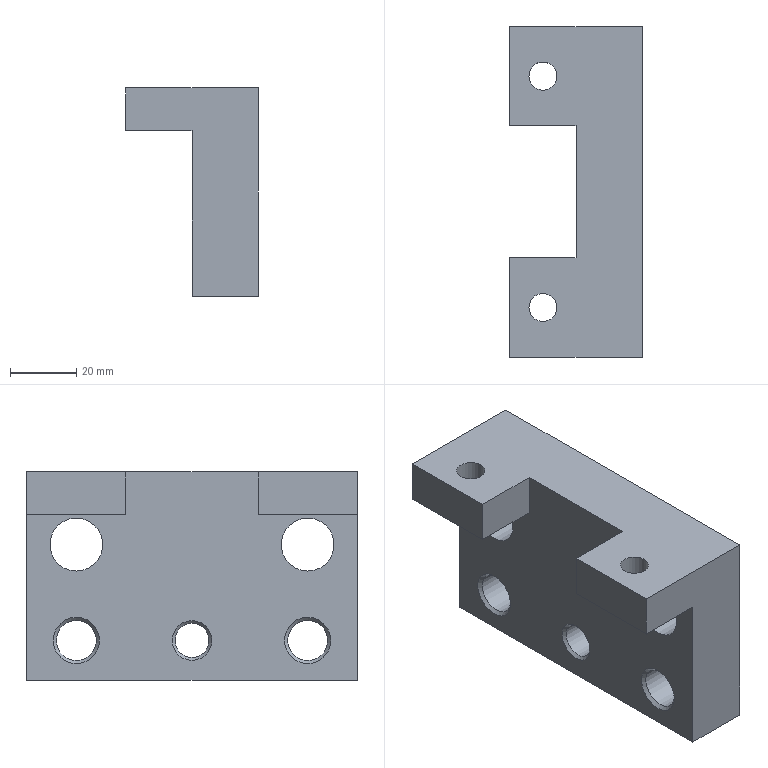Part | STEP file | Tube feed_id486_x_t | 1 solid | 29 faces | box 40 x 100 x 63 mm | volume 124553 mm3 | plane 14 | cylinder 9 | cone 6 | commonest cylinder face diameters 8.5 x2 12.1 x2 14 x2 16 x2 10.3 x1